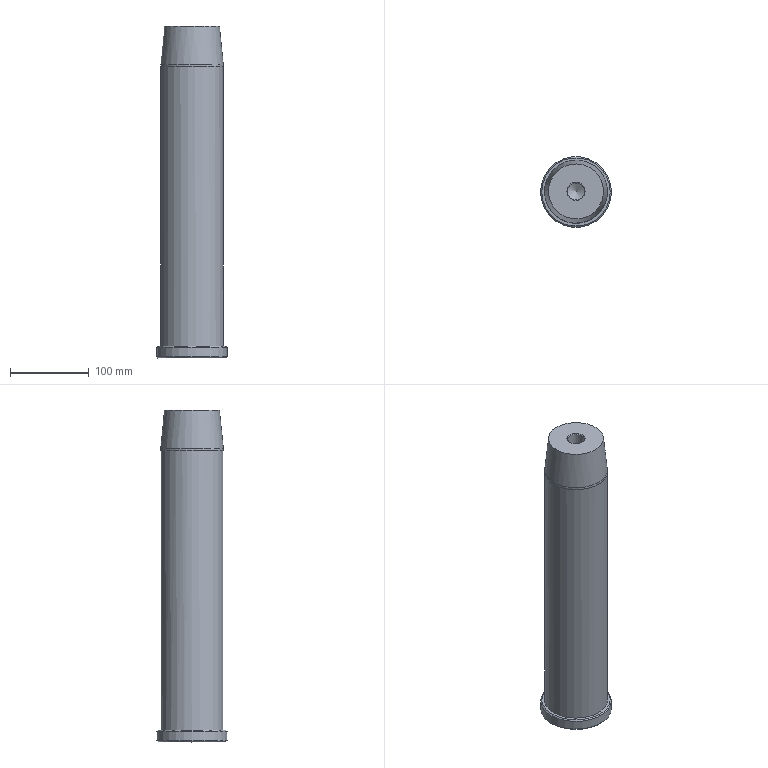Part | STEP file | solid 40 | 1 solid | 12 faces | box 90 x 90 x 422 mm | volume 2099670 mm3 | cone 4 | plane 3 | cylinder 3 | spline 2 | commonest cylinder face diameters 21 x1 80 x1 90 x1